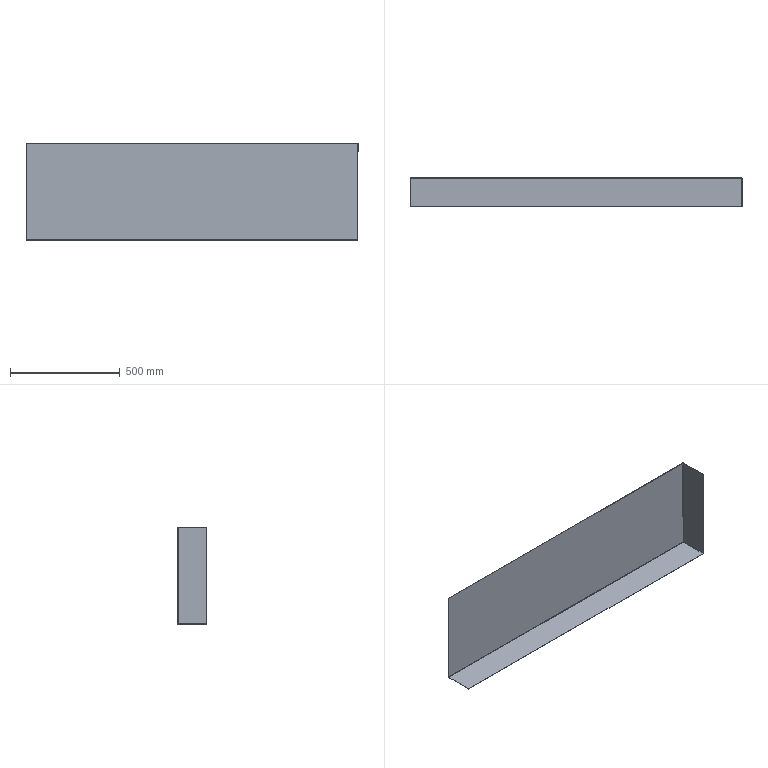Part | 1 solid | 22 faces | box 1510 x 130 x 440 mm | volume 1095979 mm3 | plane 16 | cylinder 4 | spline 2 | commonest cylinder face diameters 1.473 x2 3.873 x2
STEP:
#1=CARTESIAN_POINT('',(753.063,63.063,-1.2));
#2=VERTEX_POINT('',#1);
#3=CARTESIAN_POINT('',(753.063,-65.,-1.2));
#4=VERTEX_POINT('',#3);
#5=CARTESIAN_POINT('',(753.063,63.093,-1.2));
#6=DIRECTION('',(0.,-1.,0.));
#7=VECTOR('',#6,1000.);
#8=LINE('',#5,#7);
#9=EDGE_CURVE('',#2,#4,#8,.T.);
#10=ORIENTED_EDGE('',*,*,#9,.T.);
#11=CARTESIAN_POINT('',(-755.,-65.,-1.2));
#12=VERTEX_POINT('',#11);
#13=CARTESIAN_POINT('',(-755.,-65.,-1.2));
#14=DIRECTION('',(1.,0.,0.));
#15=VECTOR('',#14,1000.);
#16=LINE('',#13,#15);
#17=EDGE_CURVE('',#12,#4,#16,.T.);
#18=ORIENTED_EDGE('',*,*,#17,.F.);
#19=CARTESIAN_POINT('',(-755.,63.063,-1.2));
#20=VERTEX_POINT('',#19);
#21=CARTESIAN_POINT('',(-755.,65.,-1.2));
#22=DIRECTION('',(0.,-1.,0.));
#23=VECTOR('',#22,1000.);
#24=LINE('',#21,#23);
#25=EDGE_CURVE('',#20,#12,#24,.T.);
#26=ORIENTED_EDGE('',*,*,#25,.F.);
#27=CARTESIAN_POINT('',(-755.,63.063,-1.2));
#28=DIRECTION('',(1.,0.,0.));
#29=VECTOR('',#28,1000.);
#30=LINE('',#27,#29);
#31=EDGE_CURVE('',#20,#2,#30,.T.);
#32=ORIENTED_EDGE('',*,*,#31,.T.);
#33=EDGE_LOOP('',(#10,#18,#26,#32));
#34=FACE_OUTER_BOUND('',#33,.T.);
#35=CARTESIAN_POINT('',(0.,0.,-1.2));
#36=DIRECTION('',(0.,0.,1.));
#37=DIRECTION('',(1.,0.,0.));
#38=AXIS2_PLACEMENT_3D('',#35,#36,#37);
#39=PLANE('',#38);
#40=ADVANCED_FACE('',(#34),#39,.F.);
#41=CARTESIAN_POINT('',(-755.,-65.,0.));
#42=VERTEX_POINT('',#41);
#43=CARTESIAN_POINT('',(753.063,-65.,0.));
#44=VERTEX_POINT('',#43);
#45=CARTESIAN_POINT('',(-755.,-65.,0.));
#46=DIRECTION('',(1.,0.,0.));
#47=VECTOR('',#46,1000.);
#48=LINE('',#45,#47);
#49=EDGE_CURVE('',#42,#44,#48,.T.);
#50=ORIENTED_EDGE('',*,*,#49,.T.);
#51=CARTESIAN_POINT('',(753.063,63.063,0.));
#52=VERTEX_POINT('',#51);
#53=CARTESIAN_POINT('',(753.063,63.093,0.));
#54=DIRECTION('',(0.,-1.,0.));
#55=VECTOR('',#54,1000.);
#56=LINE('',#53,#55);
#57=EDGE_CURVE('',#52,#44,#56,.T.);
#58=ORIENTED_EDGE('',*,*,#57,.F.);
#59=CARTESIAN_POINT('',(-755.,63.063,0.));
#60=VERTEX_POINT('',#59);
#61=CARTESIAN_POINT('',(-755.,63.063,0.));
#62=DIRECTION('',(1.,0.,0.));
#63=VECTOR('',#62,1000.);
#64=LINE('',#61,#63);
#65=EDGE_CURVE('',#60,#52,#64,.T.);
#66=ORIENTED_EDGE('',*,*,#65,.F.);
#67=CARTESIAN_POINT('',(-755.,65.,0.));
#68=DIRECTION('',(0.,-1.,0.));
#69=VECTOR('',#68,1000.);
#70=LINE('',#67,#69);
#71=EDGE_CURVE('',#60,#42,#70,.T.);
#72=ORIENTED_EDGE('',*,*,#71,.T.);
#73=EDGE_LOOP('',(#50,#58,#66,#72));
#74=FACE_OUTER_BOUND('',#73,.T.);
#75=CARTESIAN_POINT('',(0.,0.,0.));
#76=DIRECTION('',(0.,0.,1.));
#77=DIRECTION('',(1.,0.,0.));
#78=AXIS2_PLACEMENT_3D('',#75,#76,#77);
#79=PLANE('',#78);
#80=ADVANCED_FACE('',(#74),#79,.T.);
#81=ORIENTED_EDGE('',*,*,#71,.F.);
#82=CARTESIAN_POINT('',(-755.,63.063,0.));
#83=DIRECTION('',(0.,0.,-1.));
#84=VECTOR('',#83,1000.);
#85=LINE('',#82,#84);
#86=EDGE_CURVE('',#60,#20,#85,.T.);
#87=ORIENTED_EDGE('',*,*,#86,.T.);
#88=ORIENTED_EDGE('',*,*,#25,.T.);
#89=CARTESIAN_POINT('',(-755.,-65.,-1.2));
#90=DIRECTION('',(0.,0.,1.));
#91=VECTOR('',#90,1000.);
#92=LINE('',#89,#91);
#93=EDGE_CURVE('',#12,#42,#92,.T.);
#94=ORIENTED_EDGE('',*,*,#93,.T.);
#95=EDGE_LOOP('',(#81,#87,#88,#94));
#96=FACE_OUTER_BOUND('',#95,.T.);
#97=CARTESIAN_POINT('',(-755.,65.,-1.2));
#98=DIRECTION('',(-1.,0.,0.));
#99=DIRECTION('',(0.,0.,1.));
#100=AXIS2_PLACEMENT_3D('',#97,#98,#99);
#101=PLANE('',#100);
#102=ADVANCED_FACE('',(#96),#101,.T.);
#103=CARTESIAN_POINT('',(753.063,-65.,0.));
#104=DIRECTION('',(0.,0.,-1.));
#105=VECTOR('',#104,1000.);
#106=LINE('',#103,#105);
#107=EDGE_CURVE('',#44,#4,#106,.T.);
#108=ORIENTED_EDGE('',*,*,#107,.F.);
#109=ORIENTED_EDGE('',*,*,#49,.F.);
#110=ORIENTED_EDGE('',*,*,#93,.F.);
#111=ORIENTED_EDGE('',*,*,#17,.T.);
#112=EDGE_LOOP('',(#108,#109,#110,#111));
#113=FACE_OUTER_BOUND('',#112,.T.);
#114=CARTESIAN_POINT('',(-755.,-65.,-1.2));
#115=DIRECTION('',(0.,-1.,0.));
#116=DIRECTION('',(0.,0.,-1.));
#117=AXIS2_PLACEMENT_3D('',#114,#115,#116);
#118=PLANE('',#117);
#119=ADVANCED_FACE('',(#113),#118,.T.);
#120=CARTESIAN_POINT('',(753.093,65.,0.7366));
#121=VERTEX_POINT('',#120);
#122=CARTESIAN_POINT('',(753.093,63.8,0.7366));
#123=VERTEX_POINT('',#122);
#124=CARTESIAN_POINT('',(753.093,63.8,0.7366));
#125=DIRECTION('',(0.,-1.,0.));
#126=VECTOR('',#125,1000.);
#127=LINE('',#124,#126);
#128=EDGE_CURVE('',#121,#123,#127,.T.);
#129=ORIENTED_EDGE('',*,*,#128,.T.);
#130=CARTESIAN_POINT('',(753.063,63.063,0.));
#131=CARTESIAN_POINT('',(753.068,63.256,0.));
#132=CARTESIAN_POINT('',(753.073,63.448,0.07939));
#133=CARTESIAN_POINT('',(753.083,63.721,0.3521));
#134=CARTESIAN_POINT('',(753.088,63.8,0.5438));
#135=CARTESIAN_POINT('',(753.093,63.8,0.7366));
#136=B_SPLINE_CURVE_WITH_KNOTS('',3,(#130,#131,#132,#133,#134,#135),.UNSPECIFIED.,.F.,.F.,(4,2,4),(0.,0.5,1.),.UNSPECIFIED.);
#137=EDGE_CURVE('',#52,#123,#136,.T.);
#138=ORIENTED_EDGE('',*,*,#137,.F.);
#139=CARTESIAN_POINT('',(753.063,63.063,0.));
#140=DIRECTION('',(0.,0.,-1.));
#141=VECTOR('',#140,1000.);
#142=LINE('',#139,#141);
#143=EDGE_CURVE('',#52,#2,#142,.T.);
#144=ORIENTED_EDGE('',*,*,#143,.T.);
#145=CARTESIAN_POINT('',(753.063,63.063,-1.2));
#146=CARTESIAN_POINT('',(753.066,63.317,-1.2));
#147=CARTESIAN_POINT('',(753.068,63.57,-1.15));
#148=CARTESIAN_POINT('',(753.073,64.039,-0.9556));
#149=CARTESIAN_POINT('',(753.076,64.254,-0.812));
#150=CARTESIAN_POINT('',(753.081,64.612,-0.4535));
#151=CARTESIAN_POINT('',(753.083,64.756,-0.2387));
#152=CARTESIAN_POINT('',(753.088,64.95,0.2297));
#153=CARTESIAN_POINT('',(753.09,65.,0.4831));
#154=CARTESIAN_POINT('',(753.093,65.,0.7366));
#155=B_SPLINE_CURVE_WITH_KNOTS('',3,(#145,#146,#147,#148,#149,#150,#151,#152,#153,#154),.UNSPECIFIED.,.F.,.F.,(4,2,2,2,4),(0.,0.25,0.5,0.75,1.),.UNSPECIFIED.);
#156=EDGE_CURVE('',#2,#121,#155,.T.);
#157=ORIENTED_EDGE('',*,*,#156,.T.);
#158=EDGE_LOOP('',(#129,#138,#144,#157));
#159=FACE_OUTER_BOUND('',#158,.T.);
#160=CARTESIAN_POINT('',(753.063,63.063,-1.212));
#161=CARTESIAN_POINT('',(753.066,63.319,-1.212));
#162=CARTESIAN_POINT('',(753.068,63.573,-1.161));
#163=CARTESIAN_POINT('',(753.073,64.045,-0.9661));
#164=CARTESIAN_POINT('',(753.076,64.261,-0.8216));
#165=CARTESIAN_POINT('',(753.081,64.622,-0.4609));
#166=CARTESIAN_POINT('',(753.083,64.766,-0.2448));
#167=CARTESIAN_POINT('',(753.088,64.961,0.2266));
#168=CARTESIAN_POINT('',(753.09,65.012,0.4815));
#169=CARTESIAN_POINT('',(753.093,65.012,0.7366));
#170=CARTESIAN_POINT('',(753.063,63.063,-1.2));
#171=CARTESIAN_POINT('',(753.066,63.317,-1.2));
#172=CARTESIAN_POINT('',(753.068,63.57,-1.15));
#173=CARTESIAN_POINT('',(753.073,64.039,-0.9556));
#174=CARTESIAN_POINT('',(753.076,64.254,-0.812));
#175=CARTESIAN_POINT('',(753.081,64.612,-0.4535));
#176=CARTESIAN_POINT('',(753.083,64.756,-0.2387));
#177=CARTESIAN_POINT('',(753.088,64.95,0.2297));
#178=CARTESIAN_POINT('',(753.09,65.,0.4831));
#179=CARTESIAN_POINT('',(753.093,65.,0.7366));
#180=CARTESIAN_POINT('',(753.063,63.063,0.));
#181=CARTESIAN_POINT('',(753.066,63.16,0.));
#182=CARTESIAN_POINT('',(753.068,63.256,0.01917));
#183=CARTESIAN_POINT('',(753.073,63.434,0.09297));
#184=CARTESIAN_POINT('',(753.076,63.516,0.1476));
#185=CARTESIAN_POINT('',(753.081,63.652,0.2839));
#186=CARTESIAN_POINT('',(753.083,63.707,0.3656));
#187=CARTESIAN_POINT('',(753.088,63.781,0.5438));
#188=CARTESIAN_POINT('',(753.09,63.8,0.6402));
#189=CARTESIAN_POINT('',(753.093,63.8,0.7366));
#190=CARTESIAN_POINT('',(753.063,63.063,0.01212));
#191=CARTESIAN_POINT('',(753.066,63.158,0.01212));
#192=CARTESIAN_POINT('',(753.068,63.253,0.03098));
#193=CARTESIAN_POINT('',(753.073,63.428,0.1036));
#194=CARTESIAN_POINT('',(753.076,63.509,0.1573));
#195=CARTESIAN_POINT('',(753.081,63.643,0.2914));
#196=CARTESIAN_POINT('',(753.083,63.696,0.3717));
#197=CARTESIAN_POINT('',(753.088,63.769,0.547));
#198=CARTESIAN_POINT('',(753.09,63.788,0.6417));
#199=CARTESIAN_POINT('',(753.093,63.788,0.7366));
#200=B_SPLINE_SURFACE_WITH_KNOTS('',1,3,((#160,#161,#162,#163,#164,#165,#166,#167,#168,#169),(#170,#171,#172,#173,#174,#175,#176,#177,#178,#179),(#180,#181,#182,#183,#184,#185,#186,#187,#188,#189),(#190,#191,#192,#193,#194,#195,#196,#197,#198,#199)),.UNSPECIFIED.,.F.,.F.,.F.,(2,1,1,2),(4,2,2,2,4),(-0.01,0.,1.,1.01),(0.,0.25,0.5,0.75,1.),.UNSPECIFIED.);
#201=ADVANCED_FACE('',(#159),#200,.F.);
#202=CARTESIAN_POINT('',(-755.,63.8,0.7366));
#203=VERTEX_POINT('',#202);
#204=CARTESIAN_POINT('',(-755.,63.063,0.7366));
#205=DIRECTION('',(-1.,0.,0.));
#206=DIRECTION('',(0.,0.,1.));
#207=AXIS2_PLACEMENT_3D('',#204,#205,#206);
#208=CIRCLE('',#207,0.7366);
#209=EDGE_CURVE('',#203,#60,#208,.T.);
#210=ORIENTED_EDGE('',*,*,#209,.F.);
#211=CARTESIAN_POINT('',(-755.,65.,0.7366));
#212=VERTEX_POINT('',#211);
#213=CARTESIAN_POINT('',(-755.,63.8,0.7366));
#214=DIRECTION('',(0.,1.,0.));
#215=VECTOR('',#214,1000.);
#216=LINE('',#213,#215);
#217=EDGE_CURVE('',#203,#212,#216,.T.);
#218=ORIENTED_EDGE('',*,*,#217,.T.);
#219=CARTESIAN_POINT('',(-755.,63.063,0.7366));
#220=DIRECTION('',(-1.,0.,0.));
#221=DIRECTION('',(0.,0.,1.));
#222=AXIS2_PLACEMENT_3D('',#219,#220,#221);
#223=CIRCLE('',#222,1.937);
#224=EDGE_CURVE('',#212,#20,#223,.T.);
#225=ORIENTED_EDGE('',*,*,#224,.T.);
#226=ORIENTED_EDGE('',*,*,#86,.F.);
#227=EDGE_LOOP('',(#210,#218,#225,#226));
#228=FACE_OUTER_BOUND('',#227,.T.);
#229=CARTESIAN_POINT('',(-755.,63.063,0.7366));
#230=DIRECTION('',(1.,0.,0.));
#231=DIRECTION('',(0.,0.,-1.));
#232=AXIS2_PLACEMENT_3D('',#229,#230,#231);
#233=PLANE('',#232);
#234=ADVANCED_FACE('',(#228),#233,.F.);
#235=ORIENTED_EDGE('',*,*,#31,.F.);
#236=ORIENTED_EDGE('',*,*,#224,.F.);
#237=CARTESIAN_POINT('',(0.,65.,0.7366));
#238=DIRECTION('',(-1.,0.,0.));
#239=VECTOR('',#238,1000.);
#240=LINE('',#237,#239);
#241=EDGE_CURVE('',#121,#212,#240,.T.);
#242=ORIENTED_EDGE('',*,*,#241,.F.);
#243=ORIENTED_EDGE('',*,*,#156,.F.);
#244=EDGE_LOOP('',(#235,#236,#242,#243));
#245=FACE_OUTER_BOUND('',#244,.T.);
#246=CARTESIAN_POINT('',(-755.,63.063,0.7366));
#247=DIRECTION('',(-1.,0.,0.));
#248=DIRECTION('',(0.,1.,0.));
#249=AXIS2_PLACEMENT_3D('',#246,#247,#248);
#250=CYLINDRICAL_SURFACE('',#249,1.937);
#251=ADVANCED_FACE('',(#245),#250,.T.);
#252=ORIENTED_EDGE('',*,*,#65,.T.);
#253=ORIENTED_EDGE('',*,*,#137,.T.);
#254=CARTESIAN_POINT('',(755.,63.8,0.7366));
#255=DIRECTION('',(-1.,0.,0.));
#256=VECTOR('',#255,1000.);
#257=LINE('',#254,#256);
#258=EDGE_CURVE('',#123,#203,#257,.T.);
#259=ORIENTED_EDGE('',*,*,#258,.T.);
#260=ORIENTED_EDGE('',*,*,#209,.T.);
#261=EDGE_LOOP('',(#252,#253,#259,#260));
#262=FACE_OUTER_BOUND('',#261,.T.);
#263=CARTESIAN_POINT('',(-755.,63.063,0.7366));
#264=DIRECTION('',(-1.,0.,0.));
#265=DIRECTION('',(0.,1.,0.));
#266=AXIS2_PLACEMENT_3D('',#263,#264,#265);
#267=CYLINDRICAL_SURFACE('',#266,0.7366);
#268=ADVANCED_FACE('',(#262),#267,.F.);
#269=CARTESIAN_POINT('',(753.093,63.8,438.8));
#270=VERTEX_POINT('',#269);
#271=CARTESIAN_POINT('',(753.093,65.,438.8));
#272=VERTEX_POINT('',#271);
#273=CARTESIAN_POINT('',(753.093,65.,438.8));
#274=DIRECTION('',(0.,1.,0.));
#275=VECTOR('',#274,1000.);
#276=LINE('',#273,#275);
#277=EDGE_CURVE('',#270,#272,#276,.T.);
#278=ORIENTED_EDGE('',*,*,#277,.F.);
#279=CARTESIAN_POINT('',(753.093,63.8,0.));
#280=DIRECTION('',(0.,0.,1.));
#281=VECTOR('',#280,1000.);
#282=LINE('',#279,#281);
#283=EDGE_CURVE('',#123,#270,#282,.T.);
#284=ORIENTED_EDGE('',*,*,#283,.F.);
#285=ORIENTED_EDGE('',*,*,#128,.F.);
#286=CARTESIAN_POINT('',(753.093,65.,0.));
#287=DIRECTION('',(0.,0.,-1.));
#288=VECTOR('',#287,1000.);
#289=LINE('',#286,#288);
#290=EDGE_CURVE('',#272,#121,#289,.T.);
#291=ORIENTED_EDGE('',*,*,#290,.F.);
#292=EDGE_LOOP('',(#278,#284,#285,#291));
#293=FACE_OUTER_BOUND('',#292,.T.);
#294=CARTESIAN_POINT('',(753.093,63.8,0.));
#295=DIRECTION('',(1.,0.,0.));
#296=DIRECTION('',(0.,0.,-1.));
#297=AXIS2_PLACEMENT_3D('',#294,#295,#296);
#298=PLANE('',#297);
#299=ADVANCED_FACE('',(#293),#298,.T.);
#300=CARTESIAN_POINT('',(-755.,65.,438.8));
#301=VERTEX_POINT('',#300);
#302=CARTESIAN_POINT('',(-755.,65.,438.8));
#303=DIRECTION('',(-1.,0.,0.));
#304=VECTOR('',#303,1000.);
#305=LINE('',#302,#304);
#306=EDGE_CURVE('',#272,#301,#305,.T.);
#307=ORIENTED_EDGE('',*,*,#306,.F.);
#308=ORIENTED_EDGE('',*,*,#290,.T.);
#309=ORIENTED_EDGE('',*,*,#241,.T.);
#310=CARTESIAN_POINT('',(-755.,65.,0.));
#311=DIRECTION('',(0.,0.,-1.));
#312=VECTOR('',#311,1000.);
#313=LINE('',#310,#312);
#314=EDGE_CURVE('',#301,#212,#313,.T.);
#315=ORIENTED_EDGE('',*,*,#314,.F.);
#316=EDGE_LOOP('',(#307,#308,#309,#315));
#317=FACE_OUTER_BOUND('',#316,.T.);
#318=CARTESIAN_POINT('',(0.,65.,0.));
#319=DIRECTION('',(0.,1.,0.));
#320=DIRECTION('',(0.,0.,1.));
#321=AXIS2_PLACEMENT_3D('',#318,#319,#320);
#322=PLANE('',#321);
#323=ADVANCED_FACE('',(#317),#322,.T.);
#324=ORIENTED_EDGE('',*,*,#283,.T.);
#325=CARTESIAN_POINT('',(-755.,63.8,438.8));
#326=VERTEX_POINT('',#325);
#327=CARTESIAN_POINT('',(0.,63.8,438.8));
#328=DIRECTION('',(-1.,0.,0.));
#329=VECTOR('',#328,1000.);
#330=LINE('',#327,#329);
#331=EDGE_CURVE('',#270,#326,#330,.T.);
#332=ORIENTED_EDGE('',*,*,#331,.T.);
#333=CARTESIAN_POINT('',(-755.,63.8,0.));
#334=DIRECTION('',(0.,0.,-1.));
#335=VECTOR('',#334,1000.);
#336=LINE('',#333,#335);
#337=EDGE_CURVE('',#326,#203,#336,.T.);
#338=ORIENTED_EDGE('',*,*,#337,.T.);
#339=ORIENTED_EDGE('',*,*,#258,.F.);
#340=EDGE_LOOP('',(#324,#332,#338,#339));
#341=FACE_OUTER_BOUND('',#340,.T.);
#342=CARTESIAN_POINT('',(0.,63.8,0.));
#343=DIRECTION('',(0.,1.,0.));
#344=DIRECTION('',(0.,0.,1.));
#345=AXIS2_PLACEMENT_3D('',#342,#343,#344);
#346=PLANE('',#345);
#347=ADVANCED_FACE('',(#341),#346,.F.);
#348=ORIENTED_EDGE('',*,*,#331,.F.);
#349=ORIENTED_EDGE('',*,*,#277,.T.);
#350=ORIENTED_EDGE('',*,*,#306,.T.);
#351=CARTESIAN_POINT('',(-755.,65.,438.8));
#352=DIRECTION('',(0.,-1.,0.));
#353=VECTOR('',#352,1000.);
#354=LINE('',#351,#353);
#355=EDGE_CURVE('',#301,#326,#354,.T.);
#356=ORIENTED_EDGE('',*,*,#355,.T.);
#357=EDGE_LOOP('',(#348,#349,#350,#356));
#358=FACE_OUTER_BOUND('',#357,.T.);
#359=CARTESIAN_POINT('',(-755.,65.,438.8));
#360=DIRECTION('',(0.,0.,1.));
#361=DIRECTION('',(0.,-1.,0.));
#362=AXIS2_PLACEMENT_3D('',#359,#360,#361);
#363=PLANE('',#362);
#364=ADVANCED_FACE('',(#358),#363,.T.);
#365=ORIENTED_EDGE('',*,*,#314,.T.);
#366=ORIENTED_EDGE('',*,*,#217,.F.);
#367=ORIENTED_EDGE('',*,*,#337,.F.);
#368=ORIENTED_EDGE('',*,*,#355,.F.);
#369=EDGE_LOOP('',(#365,#366,#367,#368));
#370=FACE_OUTER_BOUND('',#369,.T.);
#371=CARTESIAN_POINT('',(-755.,65.,0.));
#372=DIRECTION('',(-1.,0.,0.));
#373=DIRECTION('',(0.,0.,1.));
#374=AXIS2_PLACEMENT_3D('',#371,#372,#373);
#375=PLANE('',#374);
#376=ADVANCED_FACE('',(#370),#375,.T.);
#377=CARTESIAN_POINT('',(753.8,-65.,0.7366));
#378=VERTEX_POINT('',#377);
#379=CARTESIAN_POINT('',(755.,-65.,0.7366));
#380=VERTEX_POINT('',#379);
#381=CARTESIAN_POINT('',(755.,-65.,0.7366));
#382=DIRECTION('',(1.,0.,0.));
#383=VECTOR('',#382,1000.);
#384=LINE('',#381,#383);
#385=EDGE_CURVE('',#378,#380,#384,.T.);
#386=ORIENTED_EDGE('',*,*,#385,.F.);
#387=CARTESIAN_POINT('',(753.063,-65.,0.7366));
#388=DIRECTION('',(0.,-1.,0.));
#389=DIRECTION('',(0.,0.,1.));
#390=AXIS2_PLACEMENT_3D('',#387,#388,#389);
#391=CIRCLE('',#390,0.7366);
#392=EDGE_CURVE('',#44,#378,#391,.T.);
#393=ORIENTED_EDGE('',*,*,#392,.F.);
#394=ORIENTED_EDGE('',*,*,#107,.T.);
#395=CARTESIAN_POINT('',(753.063,-65.,0.7366));
#396=DIRECTION('',(0.,-1.,0.));
#397=DIRECTION('',(0.,0.,1.));
#398=AXIS2_PLACEMENT_3D('',#395,#396,#397);
#399=CIRCLE('',#398,1.937);
#400=EDGE_CURVE('',#4,#380,#399,.T.);
#401=ORIENTED_EDGE('',*,*,#400,.T.);
#402=EDGE_LOOP('',(#386,#393,#394,#401));
#403=FACE_OUTER_BOUND('',#402,.T.);
#404=CARTESIAN_POINT('',(753.063,-65.,0.7366));
#405=DIRECTION('',(0.,-1.,0.));
#406=DIRECTION('',(0.,0.,-1.));
#407=AXIS2_PLACEMENT_3D('',#404,#405,#406);
#408=PLANE('',#407);
#409=ADVANCED_FACE('',(#403),#408,.T.);
#410=CARTESIAN_POINT('',(753.8,63.093,0.7366));
#411=VERTEX_POINT('',#410);
#412=CARTESIAN_POINT('',(753.8,63.093,0.7366));
#413=CARTESIAN_POINT('',(753.8,63.088,0.5438));
#414=CARTESIAN_POINT('',(753.721,63.083,0.3521));
#415=CARTESIAN_POINT('',(753.448,63.073,0.07939));
#416=CARTESIAN_POINT('',(753.256,63.068,0.));
#417=CARTESIAN_POINT('',(753.063,63.063,0.));
#418=B_SPLINE_CURVE_WITH_KNOTS('',3,(#412,#413,#414,#415,#416,#417),.UNSPECIFIED.,.F.,.F.,(4,2,4),(0.,0.5,1.),.UNSPECIFIED.);
#419=EDGE_CURVE('',#411,#52,#418,.T.);
#420=ORIENTED_EDGE('',*,*,#419,.F.);
#421=CARTESIAN_POINT('',(755.,63.093,0.7366));
#422=VERTEX_POINT('',#421);
#423=CARTESIAN_POINT('',(753.8,63.093,0.7366));
#424=DIRECTION('',(-1.,0.,0.));
#425=VECTOR('',#424,1000.);
#426=LINE('',#423,#425);
#427=EDGE_CURVE('',#422,#411,#426,.T.);
#428=ORIENTED_EDGE('',*,*,#427,.F.);
#429=CARTESIAN_POINT('',(755.,63.093,0.7366));
#430=CARTESIAN_POINT('',(755.,63.09,0.4831));
#431=CARTESIAN_POINT('',(754.95,63.088,0.2297));
#432=CARTESIAN_POINT('',(754.756,63.083,-0.2387));
#433=CARTESIAN_POINT('',(754.612,63.081,-0.4535));
#434=CARTESIAN_POINT('',(754.254,63.076,-0.812));
#435=CARTESIAN_POINT('',(754.039,63.073,-0.9556));
#436=CARTESIAN_POINT('',(753.57,63.068,-1.15));
#437=CARTESIAN_POINT('',(753.317,63.066,-1.2));
#438=CARTESIAN_POINT('',(753.063,63.063,-1.2));
#439=B_SPLINE_CURVE_WITH_KNOTS('',3,(#429,#430,#431,#432,#433,#434,#435,#436,#437,#438),.UNSPECIFIED.,.F.,.F.,(4,2,2,2,4),(0.,0.25,0.5,0.75,1.),.UNSPECIFIED.);
#440=EDGE_CURVE('',#422,#2,#439,.T.);
#441=ORIENTED_EDGE('',*,*,#440,.T.);
#442=ORIENTED_EDGE('',*,*,#143,.F.);
#443=EDGE_LOOP('',(#420,#428,#441,#442));
#444=FACE_OUTER_BOUND('',#443,.T.);
#445=CARTESIAN_POINT('',(755.012,63.093,0.7366));
#446=CARTESIAN_POINT('',(755.012,63.09,0.4815));
#447=CARTESIAN_POINT('',(754.961,63.088,0.2266));
#448=CARTESIAN_POINT('',(754.766,63.083,-0.2448));
#449=CARTESIAN_POINT('',(754.622,63.081,-0.4609));
#450=CARTESIAN_POINT('',(754.261,63.076,-0.8216));
#451=CARTESIAN_POINT('',(754.045,63.073,-0.9661));
#452=CARTESIAN_POINT('',(753.573,63.068,-1.161));
#453=CARTESIAN_POINT('',(753.319,63.066,-1.212));
#454=CARTESIAN_POINT('',(753.063,63.063,-1.212));
#455=CARTESIAN_POINT('',(755.,63.093,0.7366));
#456=CARTESIAN_POINT('',(755.,63.09,0.4831));
#457=CARTESIAN_POINT('',(754.95,63.088,0.2297));
#458=CARTESIAN_POINT('',(754.756,63.083,-0.2387));
#459=CARTESIAN_POINT('',(754.612,63.081,-0.4535));
#460=CARTESIAN_POINT('',(754.254,63.076,-0.812));
#461=CARTESIAN_POINT('',(754.039,63.073,-0.9556));
#462=CARTESIAN_POINT('',(753.57,63.068,-1.15));
#463=CARTESIAN_POINT('',(753.317,63.066,-1.2));
#464=CARTESIAN_POINT('',(753.063,63.063,-1.2));
#465=CARTESIAN_POINT('',(753.8,63.093,0.7366));
#466=CARTESIAN_POINT('',(753.8,63.09,0.6402));
#467=CARTESIAN_POINT('',(753.781,63.088,0.5438));
#468=CARTESIAN_POINT('',(753.707,63.083,0.3656));
#469=CARTESIAN_POINT('',(753.652,63.081,0.2839));
#470=CARTESIAN_POINT('',(753.516,63.076,0.1476));
#471=CARTESIAN_POINT('',(753.434,63.073,0.09297));
#472=CARTESIAN_POINT('',(753.256,63.068,0.01917));
#473=CARTESIAN_POINT('',(753.16,63.066,0.));
#474=CARTESIAN_POINT('',(753.063,63.063,0.));
#475=CARTESIAN_POINT('',(753.788,63.093,0.7366));
#476=CARTESIAN_POINT('',(753.788,63.09,0.6417));
#477=CARTESIAN_POINT('',(753.769,63.088,0.547));
#478=CARTESIAN_POINT('',(753.696,63.083,0.3717));
#479=CARTESIAN_POINT('',(753.643,63.081,0.2914));
#480=CARTESIAN_POINT('',(753.509,63.076,0.1573));
#481=CARTESIAN_POINT('',(753.428,63.073,0.1036));
#482=CARTESIAN_POINT('',(753.253,63.068,0.03098));
#483=CARTESIAN_POINT('',(753.158,63.066,0.01212));
#484=CARTESIAN_POINT('',(753.063,63.063,0.01212));
#485=B_SPLINE_SURFACE_WITH_KNOTS('',1,3,((#445,#446,#447,#448,#449,#450,#451,#452,#453,#454),(#455,#456,#457,#458,#459,#460,#461,#462,#463,#464),(#465,#466,#467,#468,#469,#470,#471,#472,#473,#474),(#475,#476,#477,#478,#479,#480,#481,#482,#483,#484)),.UNSPECIFIED.,.F.,.F.,.F.,(2,1,1,2),(4,2,2,2,4),(-0.01,0.,1.,1.01),(0.,0.25,0.5,0.75,1.),.UNSPECIFIED.);
#486=ADVANCED_FACE('',(#444),#485,.F.);
#487=ORIENTED_EDGE('',*,*,#9,.F.);
#488=ORIENTED_EDGE('',*,*,#440,.F.);
#489=CARTESIAN_POINT('',(755.,-65.,0.7366));
#490=DIRECTION('',(0.,-1.,0.));
#491=VECTOR('',#490,1000.);
#492=LINE('',#489,#491);
#493=EDGE_CURVE('',#422,#380,#492,.T.);
#494=ORIENTED_EDGE('',*,*,#493,.T.);
#495=ORIENTED_EDGE('',*,*,#400,.F.);
#496=EDGE_LOOP('',(#487,#488,#494,#495));
#497=FACE_OUTER_BOUND('',#496,.T.);
#498=CARTESIAN_POINT('',(753.063,63.093,0.7366));
#499=DIRECTION('',(0.,1.,0.));
#500=DIRECTION('',(1.,0.,0.));
#501=AXIS2_PLACEMENT_3D('',#498,#499,#500);
#502=CYLINDRICAL_SURFACE('',#501,1.937);
#503=ADVANCED_FACE('',(#497),#502,.T.);
#504=ORIENTED_EDGE('',*,*,#57,.T.);
#505=ORIENTED_EDGE('',*,*,#392,.T.);
#506=CARTESIAN_POINT('',(753.8,-65.,0.7366));
#507=DIRECTION('',(0.,1.,0.));
#508=VECTOR('',#507,1000.);
#509=LINE('',#506,#508);
#510=EDGE_CURVE('',#378,#411,#509,.T.);
#511=ORIENTED_EDGE('',*,*,#510,.T.);
#512=ORIENTED_EDGE('',*,*,#419,.T.);
#513=EDGE_LOOP('',(#504,#505,#511,#512));
#514=FACE_OUTER_BOUND('',#513,.T.);
#515=CARTESIAN_POINT('',(753.063,63.093,0.7366));
#516=DIRECTION('',(0.,1.,0.));
#517=DIRECTION('',(1.,0.,0.));
#518=AXIS2_PLACEMENT_3D('',#515,#516,#517);
#519=CYLINDRICAL_SURFACE('',#518,0.7366);
#520=ADVANCED_FACE('',(#514),#519,.F.);
#521=CARTESIAN_POINT('',(753.8,-65.,438.8));
#522=VERTEX_POINT('',#521);
#523=CARTESIAN_POINT('',(753.8,-65.,0.));
#524=DIRECTION('',(0.,0.,1.));
#525=VECTOR('',#524,1000.);
#526=LINE('',#523,#525);
#527=EDGE_CURVE('',#378,#522,#526,.T.);
#528=ORIENTED_EDGE('',*,*,#527,.F.);
#529=ORIENTED_EDGE('',*,*,#385,.T.);
#530=CARTESIAN_POINT('',(755.,-65.,438.8));
#531=VERTEX_POINT('',#530);
#532=CARTESIAN_POINT('',(755.,-65.,0.));
#533=DIRECTION('',(0.,0.,1.));
#534=VECTOR('',#533,1000.);
#535=LINE('',#532,#534);
#536=EDGE_CURVE('',#380,#531,#535,.T.);
#537=ORIENTED_EDGE('',*,*,#536,.T.);
#538=CARTESIAN_POINT('',(755.,-65.,438.8));
#539=DIRECTION('',(-1.,0.,0.));
#540=VECTOR('',#539,1000.);
#541=LINE('',#538,#540);
#542=EDGE_CURVE('',#531,#522,#541,.T.);
#543=ORIENTED_EDGE('',*,*,#542,.T.);
#544=EDGE_LOOP('',(#528,#529,#537,#543));
#545=FACE_OUTER_BOUND('',#544,.T.);
#546=CARTESIAN_POINT('',(755.,-65.,0.));
#547=DIRECTION('',(0.,-1.,0.));
#548=DIRECTION('',(1.,0.,0.));
#549=AXIS2_PLACEMENT_3D('',#546,#547,#548);
#550=PLANE('',#549);
#551=ADVANCED_FACE('',(#545),#550,.T.);
#552=ORIENTED_EDGE('',*,*,#493,.F.);
#553=CARTESIAN_POINT('',(755.,63.093,438.8));
#554=VERTEX_POINT('',#553);
#555=CARTESIAN_POINT('',(755.,63.093,0.));
#556=DIRECTION('',(0.,0.,1.));
#557=VECTOR('',#556,1000.);
#558=LINE('',#555,#557);
#559=EDGE_CURVE('',#422,#554,#558,.T.);
#560=ORIENTED_EDGE('',*,*,#559,.T.);
#561=CARTESIAN_POINT('',(755.,-65.,438.8));
#562=DIRECTION('',(0.,1.,0.));
#563=VECTOR('',#562,1000.);
#564=LINE('',#561,#563);
#565=EDGE_CURVE('',#531,#554,#564,.T.);
#566=ORIENTED_EDGE('',*,*,#565,.F.);
#567=ORIENTED_EDGE('',*,*,#536,.F.);
#568=EDGE_LOOP('',(#552,#560,#566,#567));
#569=FACE_OUTER_BOUND('',#568,.T.);
#570=CARTESIAN_POINT('',(755.,0.,0.));
#571=DIRECTION('',(-1.,0.,0.));
#572=DIRECTION('',(0.,0.,1.));
#573=AXIS2_PLACEMENT_3D('',#570,#571,#572);
#574=PLANE('',#573);
#575=ADVANCED_FACE('',(#569),#574,.F.);
#576=CARTESIAN_POINT('',(753.8,63.093,438.8));
#577=VERTEX_POINT('',#576);
#578=CARTESIAN_POINT('',(753.8,63.093,0.));
#579=DIRECTION('',(0.,0.,1.));
#580=VECTOR('',#579,1000.);
#581=LINE('',#578,#580);
#582=EDGE_CURVE('',#411,#577,#581,.T.);
#583=ORIENTED_EDGE('',*,*,#582,.F.);
#584=ORIENTED_EDGE('',*,*,#510,.F.);
#585=ORIENTED_EDGE('',*,*,#527,.T.);
#586=CARTESIAN_POINT('',(753.8,0.,438.8));
#587=DIRECTION('',(0.,1.,0.));
#588=VECTOR('',#587,1000.);
#589=LINE('',#586,#588);
#590=EDGE_CURVE('',#522,#577,#589,.T.);
#591=ORIENTED_EDGE('',*,*,#590,.T.);
#592=EDGE_LOOP('',(#583,#584,#585,#591));
#593=FACE_OUTER_BOUND('',#592,.T.);
#594=CARTESIAN_POINT('',(753.8,0.,0.));
#595=DIRECTION('',(-1.,0.,0.));
#596=DIRECTION('',(0.,0.,1.));
#597=AXIS2_PLACEMENT_3D('',#594,#595,#596);
#598=PLANE('',#597);
#599=ADVANCED_FACE('',(#593),#598,.T.);
#600=CARTESIAN_POINT('',(753.8,63.093,438.8));
#601=DIRECTION('',(1.,0.,0.));
#602=VECTOR('',#601,1000.);
#603=LINE('',#600,#602);
#604=EDGE_CURVE('',#577,#554,#603,.T.);
#605=ORIENTED_EDGE('',*,*,#604,.F.);
#606=ORIENTED_EDGE('',*,*,#590,.F.);
#607=ORIENTED_EDGE('',*,*,#542,.F.);
#608=ORIENTED_EDGE('',*,*,#565,.T.);
#609=EDGE_LOOP('',(#605,#606,#607,#608));
#610=FACE_OUTER_BOUND('',#609,.T.);
#611=CARTESIAN_POINT('',(755.,-65.,438.8));
#612=DIRECTION('',(0.,0.,1.));
#613=DIRECTION('',(1.,0.,0.));
#614=AXIS2_PLACEMENT_3D('',#611,#612,#613);
#615=PLANE('',#614);
#616=ADVANCED_FACE('',(#610),#615,.T.);
#617=ORIENTED_EDGE('',*,*,#582,.T.);
#618=ORIENTED_EDGE('',*,*,#604,.T.);
#619=ORIENTED_EDGE('',*,*,#559,.F.);
#620=ORIENTED_EDGE('',*,*,#427,.T.);
#621=EDGE_LOOP('',(#617,#618,#619,#620));
#622=FACE_OUTER_BOUND('',#621,.T.);
#623=CARTESIAN_POINT('',(753.8,63.093,0.));
#624=DIRECTION('',(0.,-1.,0.));
#625=DIRECTION('',(0.,0.,-1.));
#626=AXIS2_PLACEMENT_3D('',#623,#624,#625);
#627=PLANE('',#626);
#628=ADVANCED_FACE('',(#622),#627,.F.);
#629=CLOSED_SHELL('',(#40,#80,#102,#119,#201,#234,#251,#268,#299,#323,#347,#364,#376,#409,#486,#503,#520,#551,#575,#599,#616,#628));
#630=MANIFOLD_SOLID_BREP('',#629);
#631=CARTESIAN_POINT('',(0.,0.,0.));
#632=DIRECTION('',(0.,0.,1.));
#633=DIRECTION('',(1.,0.,0.));
#634=AXIS2_PLACEMENT_3D('',#631,#632,#633);
#635=(LENGTH_UNIT()NAMED_UNIT(*)SI_UNIT(.MILLI.,.METRE.));
#636=UNCERTAINTY_MEASURE_WITH_UNIT(LENGTH_MEASURE(0.00001),#635,'','');
#637=(NAMED_UNIT(*)PLANE_ANGLE_UNIT()SI_UNIT($,.RADIAN.));
#638=(NAMED_UNIT(*)SI_UNIT($,.STERADIAN.)SOLID_ANGLE_UNIT());
#639=(GEOMETRIC_REPRESENTATION_CONTEXT(3)GLOBAL_UNCERTAINTY_ASSIGNED_CONTEXT((#636))GLOBAL_UNIT_ASSIGNED_CONTEXT((#635,#637,#638))REPRESENTATION_CONTEXT('',''));
#640=ADVANCED_BREP_SHAPE_REPRESENTATION('',(#630,#634),#639);